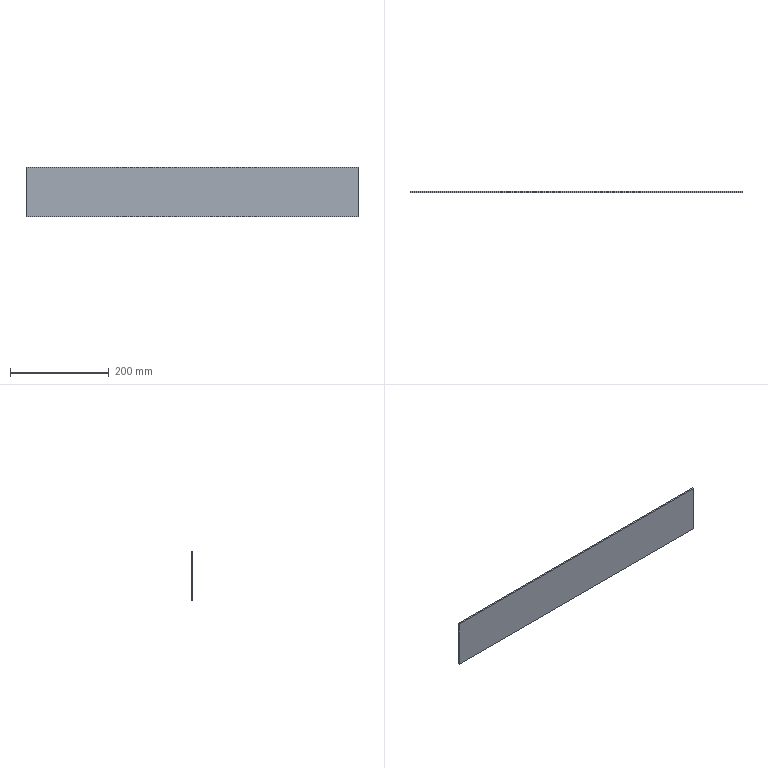Part | STEP file | Powder bin stair closing plate 1 | 1 solid | 6 faces | box 674 x 3 x 100 mm | volume 202200 mm3 | plane 6
STEP:
#1=CARTESIAN_POINT('',(0.,0.,0.));
#2=DIRECTION('',(0.,0.,1.));
#3=DIRECTION('',(1.,0.,0.));
#4=AXIS2_PLACEMENT_3D('',#1,#2,#3);
#5=CARTESIAN_POINT('',(-337.,0.,-50.));
#6=VERTEX_POINT('',#5);
#7=CARTESIAN_POINT('',(337.,0.,-50.));
#8=VERTEX_POINT('',#7);
#9=CARTESIAN_POINT('',(-337.,0.,-50.));
#10=DIRECTION('',(1.,0.,0.));
#11=VECTOR('',#10,1.);
#12=LINE('',#9,#11);
#13=CARTESIAN_POINT('',(-337.,3.,-50.));
#14=DIRECTION('',(0.,0.,-1.));
#15=DIRECTION('',(-1.,0.,0.));
#16=AXIS2_PLACEMENT_3D('',#13,#14,#15);
#17=PLANE('',#16);
#18=CARTESIAN_POINT('',(0.,-3.));
#19=DIRECTION('',(-1.,0.));
#20=VECTOR('',#19,1.);
#21=LINE('',#18,#20);
#22=(GEOMETRIC_REPRESENTATION_CONTEXT(2)PARAMETRIC_REPRESENTATION_CONTEXT()REPRESENTATION_CONTEXT('',''));
#23=DEFINITIONAL_REPRESENTATION('',(#21),#22);
#24=PCURVE('',#17,#23);
#25=CARTESIAN_POINT('',(0.,0.,0.));
#26=DIRECTION('',(0.,-1.,0.));
#27=DIRECTION('',(0.,0.,-1.));
#28=AXIS2_PLACEMENT_3D('',#25,#26,#27);
#29=PLANE('',#28);
#30=CARTESIAN_POINT('',(50.,-337.));
#31=DIRECTION('',(0.,1.));
#32=VECTOR('',#31,1.);
#33=LINE('',#30,#32);
#34=(GEOMETRIC_REPRESENTATION_CONTEXT(2)PARAMETRIC_REPRESENTATION_CONTEXT()REPRESENTATION_CONTEXT('',''));
#35=DEFINITIONAL_REPRESENTATION('',(#33),#34);
#36=PCURVE('',#29,#35);
#37=SURFACE_CURVE('',#12,(#24,#36),.PCURVE_S1.);
#38=EDGE_CURVE('',#6,#8,#37,.T.);
#39=ORIENTED_EDGE('',*,*,#38,.F.);
#40=CARTESIAN_POINT('',(-337.,3.,-50.));
#41=VERTEX_POINT('',#40);
#42=CARTESIAN_POINT('',(-337.,3.,-50.));
#43=DIRECTION('',(0.,-1.,0.));
#44=VECTOR('',#43,1.);
#45=LINE('',#42,#44);
#46=CARTESIAN_POINT('',(0.,0.));
#47=DIRECTION('',(0.,-1.));
#48=VECTOR('',#47,1.);
#49=LINE('',#46,#48);
#50=(GEOMETRIC_REPRESENTATION_CONTEXT(2)PARAMETRIC_REPRESENTATION_CONTEXT()REPRESENTATION_CONTEXT('',''));
#51=DEFINITIONAL_REPRESENTATION('',(#49),#50);
#52=PCURVE('',#17,#51);
#53=CARTESIAN_POINT('',(-337.,3.,-50.));
#54=DIRECTION('',(1.,0.,0.));
#55=DIRECTION('',(0.,0.,-1.));
#56=AXIS2_PLACEMENT_3D('',#53,#54,#55);
#57=PLANE('',#56);
#58=CARTESIAN_POINT('',(0.,0.));
#59=DIRECTION('',(0.,-1.));
#60=VECTOR('',#59,1.);
#61=LINE('',#58,#60);
#62=(GEOMETRIC_REPRESENTATION_CONTEXT(2)PARAMETRIC_REPRESENTATION_CONTEXT()REPRESENTATION_CONTEXT('',''));
#63=DEFINITIONAL_REPRESENTATION('',(#61),#62);
#64=PCURVE('',#57,#63);
#65=SURFACE_CURVE('',#45,(#52,#64),.PCURVE_S1.);
#66=EDGE_CURVE('',#41,#6,#65,.T.);
#67=ORIENTED_EDGE('',*,*,#66,.F.);
#68=CARTESIAN_POINT('',(337.,3.,-50.));
#69=VERTEX_POINT('',#68);
#70=CARTESIAN_POINT('',(-337.,3.,-50.));
#71=DIRECTION('',(1.,0.,0.));
#72=VECTOR('',#71,1.);
#73=LINE('',#70,#72);
#74=CARTESIAN_POINT('',(0.,0.));
#75=DIRECTION('',(-1.,0.));
#76=VECTOR('',#75,1.);
#77=LINE('',#74,#76);
#78=(GEOMETRIC_REPRESENTATION_CONTEXT(2)PARAMETRIC_REPRESENTATION_CONTEXT()REPRESENTATION_CONTEXT('',''));
#79=DEFINITIONAL_REPRESENTATION('',(#77),#78);
#80=PCURVE('',#17,#79);
#81=CARTESIAN_POINT('',(0.,3.,0.));
#82=DIRECTION('',(0.,-1.,0.));
#83=DIRECTION('',(0.,0.,-1.));
#84=AXIS2_PLACEMENT_3D('',#81,#82,#83);
#85=PLANE('',#84);
#86=CARTESIAN_POINT('',(50.,-337.));
#87=DIRECTION('',(0.,1.));
#88=VECTOR('',#87,1.);
#89=LINE('',#86,#88);
#90=(GEOMETRIC_REPRESENTATION_CONTEXT(2)PARAMETRIC_REPRESENTATION_CONTEXT()REPRESENTATION_CONTEXT('',''));
#91=DEFINITIONAL_REPRESENTATION('',(#89),#90);
#92=PCURVE('',#85,#91);
#93=SURFACE_CURVE('',#73,(#80,#92),.PCURVE_S1.);
#94=EDGE_CURVE('',#41,#69,#93,.T.);
#95=ORIENTED_EDGE('',*,*,#94,.T.);
#96=CARTESIAN_POINT('',(337.,3.,-50.));
#97=DIRECTION('',(0.,-1.,0.));
#98=VECTOR('',#97,1.);
#99=LINE('',#96,#98);
#100=CARTESIAN_POINT('',(-674.,0.));
#101=DIRECTION('',(0.,-1.));
#102=VECTOR('',#101,1.);
#103=LINE('',#100,#102);
#104=(GEOMETRIC_REPRESENTATION_CONTEXT(2)PARAMETRIC_REPRESENTATION_CONTEXT()REPRESENTATION_CONTEXT('',''));
#105=DEFINITIONAL_REPRESENTATION('',(#103),#104);
#106=PCURVE('',#17,#105);
#107=CARTESIAN_POINT('',(337.,3.,-50.));
#108=DIRECTION('',(1.,0.,0.));
#109=DIRECTION('',(0.,0.,-1.));
#110=AXIS2_PLACEMENT_3D('',#107,#108,#109);
#111=PLANE('',#110);
#112=CARTESIAN_POINT('',(0.,0.));
#113=DIRECTION('',(0.,-1.));
#114=VECTOR('',#113,1.);
#115=LINE('',#112,#114);
#116=(GEOMETRIC_REPRESENTATION_CONTEXT(2)PARAMETRIC_REPRESENTATION_CONTEXT()REPRESENTATION_CONTEXT('',''));
#117=DEFINITIONAL_REPRESENTATION('',(#115),#116);
#118=PCURVE('',#111,#117);
#119=SURFACE_CURVE('',#99,(#106,#118),.PCURVE_S1.);
#120=EDGE_CURVE('',#69,#8,#119,.T.);
#121=ORIENTED_EDGE('',*,*,#120,.T.);
#122=EDGE_LOOP('',(#39,#67,#95,#121));
#123=FACE_BOUND('',#122,.T.);
#124=ADVANCED_FACE('',(#123),#17,.T.);
#125=CARTESIAN_POINT('',(-337.,0.,50.));
#126=VERTEX_POINT('',#125);
#127=CARTESIAN_POINT('',(-337.,0.,-50.));
#128=DIRECTION('',(0.,0.,1.));
#129=VECTOR('',#128,1.);
#130=LINE('',#127,#129);
#131=CARTESIAN_POINT('',(0.,-3.));
#132=DIRECTION('',(-1.,0.));
#133=VECTOR('',#132,1.);
#134=LINE('',#131,#133);
#135=(GEOMETRIC_REPRESENTATION_CONTEXT(2)PARAMETRIC_REPRESENTATION_CONTEXT()REPRESENTATION_CONTEXT('',''));
#136=DEFINITIONAL_REPRESENTATION('',(#134),#135);
#137=PCURVE('',#57,#136);
#138=CARTESIAN_POINT('',(50.,-337.));
#139=DIRECTION('',(-1.,0.));
#140=VECTOR('',#139,1.);
#141=LINE('',#138,#140);
#142=(GEOMETRIC_REPRESENTATION_CONTEXT(2)PARAMETRIC_REPRESENTATION_CONTEXT()REPRESENTATION_CONTEXT('',''));
#143=DEFINITIONAL_REPRESENTATION('',(#141),#142);
#144=PCURVE('',#29,#143);
#145=SURFACE_CURVE('',#130,(#137,#144),.PCURVE_S1.);
#146=EDGE_CURVE('',#6,#126,#145,.T.);
#147=ORIENTED_EDGE('',*,*,#146,.T.);
#148=CARTESIAN_POINT('',(-337.,3.,50.));
#149=VERTEX_POINT('',#148);
#150=CARTESIAN_POINT('',(-337.,3.,50.));
#151=DIRECTION('',(0.,-1.,0.));
#152=VECTOR('',#151,1.);
#153=LINE('',#150,#152);
#154=CARTESIAN_POINT('',(-100.,0.));
#155=DIRECTION('',(0.,-1.));
#156=VECTOR('',#155,1.);
#157=LINE('',#154,#156);
#158=(GEOMETRIC_REPRESENTATION_CONTEXT(2)PARAMETRIC_REPRESENTATION_CONTEXT()REPRESENTATION_CONTEXT('',''));
#159=DEFINITIONAL_REPRESENTATION('',(#157),#158);
#160=PCURVE('',#57,#159);
#161=CARTESIAN_POINT('',(-337.,3.,50.));
#162=DIRECTION('',(0.,0.,-1.));
#163=DIRECTION('',(-1.,0.,0.));
#164=AXIS2_PLACEMENT_3D('',#161,#162,#163);
#165=PLANE('',#164);
#166=CARTESIAN_POINT('',(0.,0.));
#167=DIRECTION('',(0.,-1.));
#168=VECTOR('',#167,1.);
#169=LINE('',#166,#168);
#170=(GEOMETRIC_REPRESENTATION_CONTEXT(2)PARAMETRIC_REPRESENTATION_CONTEXT()REPRESENTATION_CONTEXT('',''));
#171=DEFINITIONAL_REPRESENTATION('',(#169),#170);
#172=PCURVE('',#165,#171);
#173=SURFACE_CURVE('',#153,(#160,#172),.PCURVE_S1.);
#174=EDGE_CURVE('',#149,#126,#173,.T.);
#175=ORIENTED_EDGE('',*,*,#174,.F.);
#176=CARTESIAN_POINT('',(-337.,3.,-50.));
#177=DIRECTION('',(0.,0.,1.));
#178=VECTOR('',#177,1.);
#179=LINE('',#176,#178);
#180=CARTESIAN_POINT('',(0.,0.));
#181=DIRECTION('',(-1.,0.));
#182=VECTOR('',#181,1.);
#183=LINE('',#180,#182);
#184=(GEOMETRIC_REPRESENTATION_CONTEXT(2)PARAMETRIC_REPRESENTATION_CONTEXT()REPRESENTATION_CONTEXT('',''));
#185=DEFINITIONAL_REPRESENTATION('',(#183),#184);
#186=PCURVE('',#57,#185);
#187=CARTESIAN_POINT('',(50.,-337.));
#188=DIRECTION('',(-1.,0.));
#189=VECTOR('',#188,1.);
#190=LINE('',#187,#189);
#191=(GEOMETRIC_REPRESENTATION_CONTEXT(2)PARAMETRIC_REPRESENTATION_CONTEXT()REPRESENTATION_CONTEXT('',''));
#192=DEFINITIONAL_REPRESENTATION('',(#190),#191);
#193=PCURVE('',#85,#192);
#194=SURFACE_CURVE('',#179,(#186,#193),.PCURVE_S1.);
#195=EDGE_CURVE('',#41,#149,#194,.T.);
#196=ORIENTED_EDGE('',*,*,#195,.F.);
#197=ORIENTED_EDGE('',*,*,#66,.T.);
#198=EDGE_LOOP('',(#147,#175,#196,#197));
#199=FACE_BOUND('',#198,.T.);
#200=ADVANCED_FACE('',(#199),#57,.F.);
#201=CARTESIAN_POINT('',(337.,0.,50.));
#202=VERTEX_POINT('',#201);
#203=CARTESIAN_POINT('',(-337.,0.,50.));
#204=DIRECTION('',(1.,0.,0.));
#205=VECTOR('',#204,1.);
#206=LINE('',#203,#205);
#207=CARTESIAN_POINT('',(0.,-3.));
#208=DIRECTION('',(-1.,0.));
#209=VECTOR('',#208,1.);
#210=LINE('',#207,#209);
#211=(GEOMETRIC_REPRESENTATION_CONTEXT(2)PARAMETRIC_REPRESENTATION_CONTEXT()REPRESENTATION_CONTEXT('',''));
#212=DEFINITIONAL_REPRESENTATION('',(#210),#211);
#213=PCURVE('',#165,#212);
#214=CARTESIAN_POINT('',(-50.,-337.));
#215=DIRECTION('',(0.,1.));
#216=VECTOR('',#215,1.);
#217=LINE('',#214,#216);
#218=(GEOMETRIC_REPRESENTATION_CONTEXT(2)PARAMETRIC_REPRESENTATION_CONTEXT()REPRESENTATION_CONTEXT('',''));
#219=DEFINITIONAL_REPRESENTATION('',(#217),#218);
#220=PCURVE('',#29,#219);
#221=SURFACE_CURVE('',#206,(#213,#220),.PCURVE_S1.);
#222=EDGE_CURVE('',#126,#202,#221,.T.);
#223=ORIENTED_EDGE('',*,*,#222,.T.);
#224=CARTESIAN_POINT('',(337.,3.,50.));
#225=VERTEX_POINT('',#224);
#226=CARTESIAN_POINT('',(337.,3.,50.));
#227=DIRECTION('',(0.,-1.,0.));
#228=VECTOR('',#227,1.);
#229=LINE('',#226,#228);
#230=CARTESIAN_POINT('',(-674.,0.));
#231=DIRECTION('',(0.,-1.));
#232=VECTOR('',#231,1.);
#233=LINE('',#230,#232);
#234=(GEOMETRIC_REPRESENTATION_CONTEXT(2)PARAMETRIC_REPRESENTATION_CONTEXT()REPRESENTATION_CONTEXT('',''));
#235=DEFINITIONAL_REPRESENTATION('',(#233),#234);
#236=PCURVE('',#165,#235);
#237=CARTESIAN_POINT('',(-100.,0.));
#238=DIRECTION('',(0.,-1.));
#239=VECTOR('',#238,1.);
#240=LINE('',#237,#239);
#241=(GEOMETRIC_REPRESENTATION_CONTEXT(2)PARAMETRIC_REPRESENTATION_CONTEXT()REPRESENTATION_CONTEXT('',''));
#242=DEFINITIONAL_REPRESENTATION('',(#240),#241);
#243=PCURVE('',#111,#242);
#244=SURFACE_CURVE('',#229,(#236,#243),.PCURVE_S1.);
#245=EDGE_CURVE('',#225,#202,#244,.T.);
#246=ORIENTED_EDGE('',*,*,#245,.F.);
#247=CARTESIAN_POINT('',(-337.,3.,50.));
#248=DIRECTION('',(1.,0.,0.));
#249=VECTOR('',#248,1.);
#250=LINE('',#247,#249);
#251=CARTESIAN_POINT('',(0.,0.));
#252=DIRECTION('',(-1.,0.));
#253=VECTOR('',#252,1.);
#254=LINE('',#251,#253);
#255=(GEOMETRIC_REPRESENTATION_CONTEXT(2)PARAMETRIC_REPRESENTATION_CONTEXT()REPRESENTATION_CONTEXT('',''));
#256=DEFINITIONAL_REPRESENTATION('',(#254),#255);
#257=PCURVE('',#165,#256);
#258=CARTESIAN_POINT('',(-50.,-337.));
#259=DIRECTION('',(0.,1.));
#260=VECTOR('',#259,1.);
#261=LINE('',#258,#260);
#262=(GEOMETRIC_REPRESENTATION_CONTEXT(2)PARAMETRIC_REPRESENTATION_CONTEXT()REPRESENTATION_CONTEXT('',''));
#263=DEFINITIONAL_REPRESENTATION('',(#261),#262);
#264=PCURVE('',#85,#263);
#265=SURFACE_CURVE('',#250,(#257,#264),.PCURVE_S1.);
#266=EDGE_CURVE('',#149,#225,#265,.T.);
#267=ORIENTED_EDGE('',*,*,#266,.F.);
#268=ORIENTED_EDGE('',*,*,#174,.T.);
#269=EDGE_LOOP('',(#223,#246,#267,#268));
#270=FACE_BOUND('',#269,.T.);
#271=ADVANCED_FACE('',(#270),#165,.F.);
#272=CARTESIAN_POINT('',(337.,0.,-50.));
#273=DIRECTION('',(0.,0.,1.));
#274=VECTOR('',#273,1.);
#275=LINE('',#272,#274);
#276=CARTESIAN_POINT('',(0.,-3.));
#277=DIRECTION('',(-1.,0.));
#278=VECTOR('',#277,1.);
#279=LINE('',#276,#278);
#280=(GEOMETRIC_REPRESENTATION_CONTEXT(2)PARAMETRIC_REPRESENTATION_CONTEXT()REPRESENTATION_CONTEXT('',''));
#281=DEFINITIONAL_REPRESENTATION('',(#279),#280);
#282=PCURVE('',#111,#281);
#283=CARTESIAN_POINT('',(50.,337.));
#284=DIRECTION('',(-1.,0.));
#285=VECTOR('',#284,1.);
#286=LINE('',#283,#285);
#287=(GEOMETRIC_REPRESENTATION_CONTEXT(2)PARAMETRIC_REPRESENTATION_CONTEXT()REPRESENTATION_CONTEXT('',''));
#288=DEFINITIONAL_REPRESENTATION('',(#286),#287);
#289=PCURVE('',#29,#288);
#290=SURFACE_CURVE('',#275,(#282,#289),.PCURVE_S1.);
#291=EDGE_CURVE('',#8,#202,#290,.T.);
#292=ORIENTED_EDGE('',*,*,#291,.F.);
#293=ORIENTED_EDGE('',*,*,#120,.F.);
#294=CARTESIAN_POINT('',(337.,3.,-50.));
#295=DIRECTION('',(0.,0.,1.));
#296=VECTOR('',#295,1.);
#297=LINE('',#294,#296);
#298=CARTESIAN_POINT('',(0.,0.));
#299=DIRECTION('',(-1.,0.));
#300=VECTOR('',#299,1.);
#301=LINE('',#298,#300);
#302=(GEOMETRIC_REPRESENTATION_CONTEXT(2)PARAMETRIC_REPRESENTATION_CONTEXT()REPRESENTATION_CONTEXT('',''));
#303=DEFINITIONAL_REPRESENTATION('',(#301),#302);
#304=PCURVE('',#111,#303);
#305=CARTESIAN_POINT('',(50.,337.));
#306=DIRECTION('',(-1.,0.));
#307=VECTOR('',#306,1.);
#308=LINE('',#305,#307);
#309=(GEOMETRIC_REPRESENTATION_CONTEXT(2)PARAMETRIC_REPRESENTATION_CONTEXT()REPRESENTATION_CONTEXT('',''));
#310=DEFINITIONAL_REPRESENTATION('',(#308),#309);
#311=PCURVE('',#85,#310);
#312=SURFACE_CURVE('',#297,(#304,#311),.PCURVE_S1.);
#313=EDGE_CURVE('',#69,#225,#312,.T.);
#314=ORIENTED_EDGE('',*,*,#313,.T.);
#315=ORIENTED_EDGE('',*,*,#245,.T.);
#316=EDGE_LOOP('',(#292,#293,#314,#315));
#317=FACE_BOUND('',#316,.T.);
#318=ADVANCED_FACE('',(#317),#111,.T.);
#319=ORIENTED_EDGE('',*,*,#94,.F.);
#320=ORIENTED_EDGE('',*,*,#195,.T.);
#321=ORIENTED_EDGE('',*,*,#266,.T.);
#322=ORIENTED_EDGE('',*,*,#313,.F.);
#323=EDGE_LOOP('',(#319,#320,#321,#322));
#324=FACE_BOUND('',#323,.T.);
#325=ADVANCED_FACE('',(#324),#85,.F.);
#326=ORIENTED_EDGE('',*,*,#38,.T.);
#327=ORIENTED_EDGE('',*,*,#291,.T.);
#328=ORIENTED_EDGE('',*,*,#222,.F.);
#329=ORIENTED_EDGE('',*,*,#146,.F.);
#330=EDGE_LOOP('',(#326,#327,#328,#329));
#331=FACE_BOUND('',#330,.T.);
#332=ADVANCED_FACE('',(#331),#29,.T.);
#333=CLOSED_SHELL('',(#124,#200,#271,#318,#325,#332));
#334=MANIFOLD_SOLID_BREP('',#333);
#335=(LENGTH_UNIT()NAMED_UNIT(*)SI_UNIT(.MILLI.,.METRE.));
#336=UNCERTAINTY_MEASURE_WITH_UNIT(LENGTH_MEASURE(0.0000001),#335,'','');
#337=(NAMED_UNIT(*)PLANE_ANGLE_UNIT()SI_UNIT($,.RADIAN.));
#338=(NAMED_UNIT(*)SI_UNIT($,.STERADIAN.)SOLID_ANGLE_UNIT());
#339=(GEOMETRIC_REPRESENTATION_CONTEXT(3)GLOBAL_UNCERTAINTY_ASSIGNED_CONTEXT((#336))GLOBAL_UNIT_ASSIGNED_CONTEXT((#335,#337,#338))REPRESENTATION_CONTEXT('',''));
#340=ADVANCED_BREP_SHAPE_REPRESENTATION('',(#4,#334),#339);